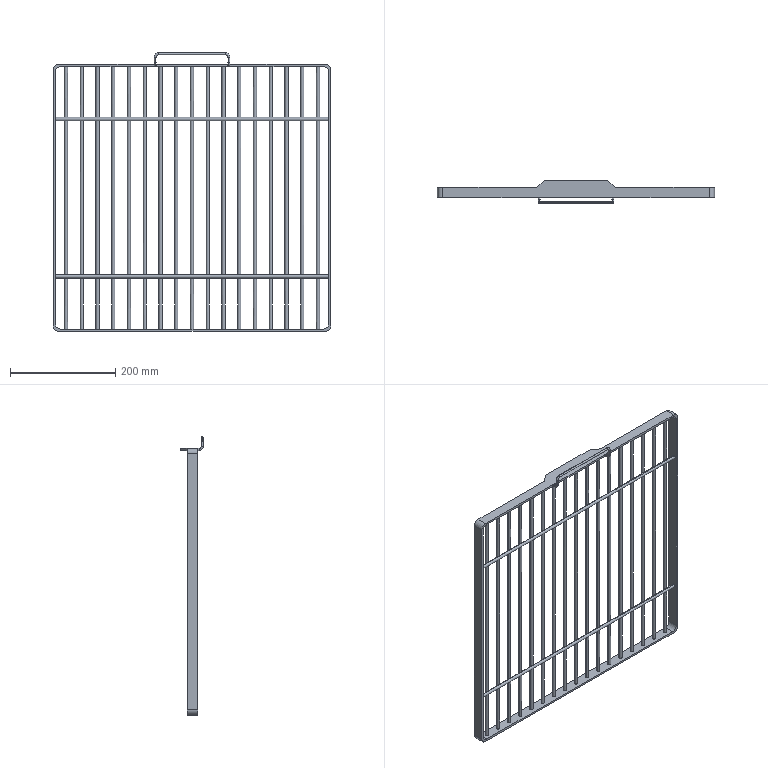Part | SolidWorks | features ICE 3, LPattern 2, Sweep 2, Extrusion 1, Fillet 1, MirrorPattern 1 | 1 solid | 78 faces | box 528 x 43 x 530 mm | volume 442043 mm3 | cylinder 56 | plane 14 | torus 8 | commonest cylinder face diameters 6 x38 4 x10 20 x8